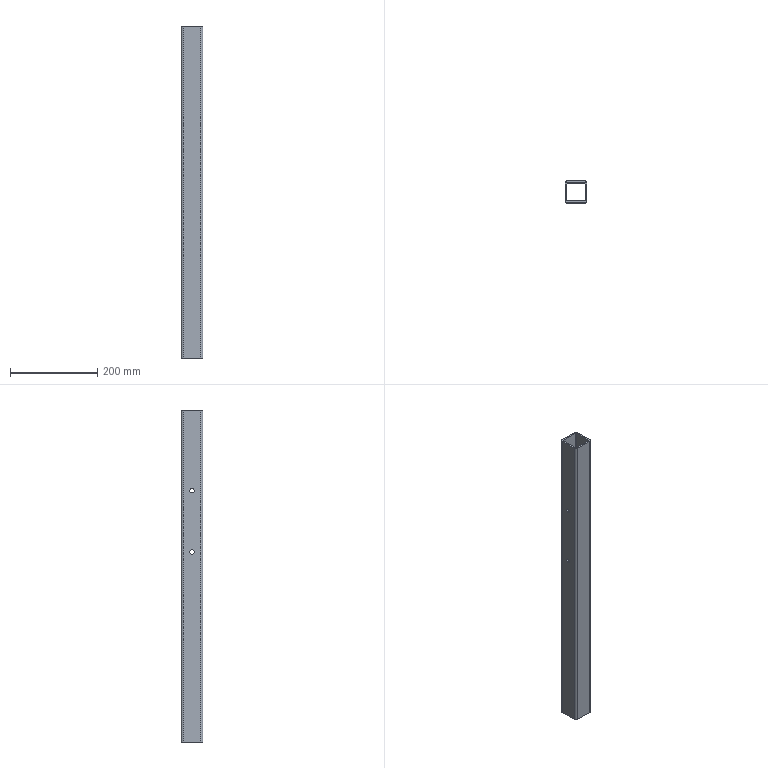Part | STEP file | 冲床-300配套压波_id1142_x_t | 1 solid | 22 faces | box 50 x 50 x 760 mm | volume 542446 mm3 | cylinder 12 | plane 10 | commonest cylinder face diameters 10 x8 2 x4
STEP:
#1=CARTESIAN_POINT('',(1916.,235.,-20.));
#2=VERTEX_POINT('',#1);
#3=CARTESIAN_POINT('',(1916.,275.,-20.));
#4=VERTEX_POINT('',#3);
#5=CARTESIAN_POINT('',(1916.,30.,-20.));
#6=DIRECTION('',(0.,1.,0.));
#7=VECTOR('',#6,1.);
#8=LINE('',#5,#7);
#9=EDGE_CURVE('',#2,#4,#8,.T.);
#10=ORIENTED_EDGE('',*,*,#9,.F.);
#11=CARTESIAN_POINT('',(1915.,234.,-20.));
#12=VERTEX_POINT('',#11);
#13=CARTESIAN_POINT('',(1915.,235.,-20.));
#14=DIRECTION('',(0.,0.,1.));
#15=DIRECTION('',(-1.,0.,0.));
#16=AXIS2_PLACEMENT_3D('',#13,#14,#15);
#17=CIRCLE('',#16,1.);
#18=EDGE_CURVE('',#12,#2,#17,.T.);
#19=ORIENTED_EDGE('',*,*,#18,.F.);
#20=CARTESIAN_POINT('',(1875.,234.,-20.));
#21=VERTEX_POINT('',#20);
#22=CARTESIAN_POINT('',(3070.,234.,-20.));
#23=DIRECTION('',(1.,0.,0.));
#24=VECTOR('',#23,1.);
#25=LINE('',#22,#24);
#26=EDGE_CURVE('',#21,#12,#25,.T.);
#27=ORIENTED_EDGE('',*,*,#26,.F.);
#28=CARTESIAN_POINT('',(1874.,235.,-20.));
#29=VERTEX_POINT('',#28);
#30=CARTESIAN_POINT('',(1875.,235.,-20.));
#31=DIRECTION('',(0.,0.,1.));
#32=DIRECTION('',(-1.,0.,0.));
#33=AXIS2_PLACEMENT_3D('',#30,#31,#32);
#34=CIRCLE('',#33,1.);
#35=EDGE_CURVE('',#29,#21,#34,.T.);
#36=ORIENTED_EDGE('',*,*,#35,.F.);
#37=CARTESIAN_POINT('',(1874.,275.,-20.));
#38=VERTEX_POINT('',#37);
#39=CARTESIAN_POINT('',(1874.,30.,-20.));
#40=DIRECTION('',(0.,-1.,0.));
#41=VECTOR('',#40,1.);
#42=LINE('',#39,#41);
#43=EDGE_CURVE('',#38,#29,#42,.T.);
#44=ORIENTED_EDGE('',*,*,#43,.F.);
#45=CARTESIAN_POINT('',(1875.,276.,-20.));
#46=VERTEX_POINT('',#45);
#47=CARTESIAN_POINT('',(1875.,275.,-20.));
#48=DIRECTION('',(0.,0.,1.));
#49=DIRECTION('',(-1.,0.,0.));
#50=AXIS2_PLACEMENT_3D('',#47,#48,#49);
#51=CIRCLE('',#50,1.);
#52=EDGE_CURVE('',#46,#38,#51,.T.);
#53=ORIENTED_EDGE('',*,*,#52,.F.);
#54=CARTESIAN_POINT('',(1915.,276.,-20.));
#55=VERTEX_POINT('',#54);
#56=CARTESIAN_POINT('',(3070.,276.,-20.));
#57=DIRECTION('',(-1.,0.,0.));
#58=VECTOR('',#57,1.);
#59=LINE('',#56,#58);
#60=EDGE_CURVE('',#55,#46,#59,.T.);
#61=ORIENTED_EDGE('',*,*,#60,.F.);
#62=CARTESIAN_POINT('',(1915.,275.,-20.));
#63=DIRECTION('',(0.,0.,1.));
#64=DIRECTION('',(-1.,0.,0.));
#65=AXIS2_PLACEMENT_3D('',#62,#63,#64);
#66=CIRCLE('',#65,1.);
#67=EDGE_CURVE('',#4,#55,#66,.T.);
#68=ORIENTED_EDGE('',*,*,#67,.F.);
#69=EDGE_LOOP('',(#10,#19,#27,#36,#44,#53,#61,#68));
#70=FACE_BOUND('',#69,.T.);
#71=CARTESIAN_POINT('',(1920.,235.,-20.));
#72=VERTEX_POINT('',#71);
#73=CARTESIAN_POINT('',(1920.,275.,-20.));
#74=VERTEX_POINT('',#73);
#75=CARTESIAN_POINT('',(1920.,275.,-20.));
#76=DIRECTION('',(0.,1.,0.));
#77=VECTOR('',#76,1.);
#78=LINE('',#75,#77);
#79=EDGE_CURVE('',#72,#74,#78,.T.);
#80=ORIENTED_EDGE('',*,*,#79,.T.);
#81=CARTESIAN_POINT('',(1915.,280.,-20.));
#82=VERTEX_POINT('',#81);
#83=CARTESIAN_POINT('',(1915.,275.,-20.));
#84=DIRECTION('',(0.,0.,1.));
#85=DIRECTION('',(-1.,0.,0.));
#86=AXIS2_PLACEMENT_3D('',#83,#84,#85);
#87=CIRCLE('',#86,5.);
#88=EDGE_CURVE('',#74,#82,#87,.T.);
#89=ORIENTED_EDGE('',*,*,#88,.T.);
#90=CARTESIAN_POINT('',(1875.,280.,-20.));
#91=VERTEX_POINT('',#90);
#92=CARTESIAN_POINT('',(1875.,280.,-20.));
#93=DIRECTION('',(-1.,0.,0.));
#94=VECTOR('',#93,1.);
#95=LINE('',#92,#94);
#96=EDGE_CURVE('',#82,#91,#95,.T.);
#97=ORIENTED_EDGE('',*,*,#96,.T.);
#98=CARTESIAN_POINT('',(1870.,275.,-20.));
#99=VERTEX_POINT('',#98);
#100=CARTESIAN_POINT('',(1875.,275.,-20.));
#101=DIRECTION('',(0.,0.,1.));
#102=DIRECTION('',(-1.,0.,0.));
#103=AXIS2_PLACEMENT_3D('',#100,#101,#102);
#104=CIRCLE('',#103,5.);
#105=EDGE_CURVE('',#91,#99,#104,.T.);
#106=ORIENTED_EDGE('',*,*,#105,.T.);
#107=CARTESIAN_POINT('',(1870.,235.,-20.));
#108=VERTEX_POINT('',#107);
#109=CARTESIAN_POINT('',(1870.,235.,-20.));
#110=DIRECTION('',(0.,-1.,0.));
#111=VECTOR('',#110,1.);
#112=LINE('',#109,#111);
#113=EDGE_CURVE('',#99,#108,#112,.T.);
#114=ORIENTED_EDGE('',*,*,#113,.T.);
#115=CARTESIAN_POINT('',(1875.,230.,-20.));
#116=VERTEX_POINT('',#115);
#117=CARTESIAN_POINT('',(1875.,235.,-20.));
#118=DIRECTION('',(0.,0.,1.));
#119=DIRECTION('',(-1.,0.,0.));
#120=AXIS2_PLACEMENT_3D('',#117,#118,#119);
#121=CIRCLE('',#120,5.);
#122=EDGE_CURVE('',#108,#116,#121,.T.);
#123=ORIENTED_EDGE('',*,*,#122,.T.);
#124=CARTESIAN_POINT('',(1915.,230.,-20.));
#125=VERTEX_POINT('',#124);
#126=CARTESIAN_POINT('',(1915.,230.,-20.));
#127=DIRECTION('',(1.,0.,0.));
#128=VECTOR('',#127,1.);
#129=LINE('',#126,#128);
#130=EDGE_CURVE('',#116,#125,#129,.T.);
#131=ORIENTED_EDGE('',*,*,#130,.T.);
#132=CARTESIAN_POINT('',(1915.,235.,-20.));
#133=DIRECTION('',(0.,0.,1.));
#134=DIRECTION('',(-1.,0.,0.));
#135=AXIS2_PLACEMENT_3D('',#132,#133,#134);
#136=CIRCLE('',#135,5.);
#137=EDGE_CURVE('',#125,#72,#136,.T.);
#138=ORIENTED_EDGE('',*,*,#137,.T.);
#139=EDGE_LOOP('',(#80,#89,#97,#106,#114,#123,#131,#138));
#140=FACE_BOUND('',#139,.T.);
#141=CARTESIAN_POINT('',(3070.,30.,-20.));
#142=DIRECTION('',(0.,0.,1.));
#143=DIRECTION('',(-1.,0.,0.));
#144=AXIS2_PLACEMENT_3D('',#141,#142,#143);
#145=PLANE('',#144);
#146=ADVANCED_FACE('',(#70,#140),#145,.T.);
#147=CARTESIAN_POINT('',(1915.,230.,-780.));
#148=VERTEX_POINT('',#147);
#149=CARTESIAN_POINT('',(1915.,230.,-740.));
#150=DIRECTION('',(0.,0.,-1.));
#151=VECTOR('',#150,1.);
#152=LINE('',#149,#151);
#153=EDGE_CURVE('',#125,#148,#152,.T.);
#154=ORIENTED_EDGE('',*,*,#153,.T.);
#155=CARTESIAN_POINT('',(1920.,235.,-780.));
#156=VERTEX_POINT('',#155);
#157=CARTESIAN_POINT('',(1915.,235.,-780.));
#158=DIRECTION('',(0.,0.,1.));
#159=DIRECTION('',(-1.,0.,0.));
#160=AXIS2_PLACEMENT_3D('',#157,#158,#159);
#161=CIRCLE('',#160,5.);
#162=EDGE_CURVE('',#148,#156,#161,.T.);
#163=ORIENTED_EDGE('',*,*,#162,.T.);
#164=CARTESIAN_POINT('',(1920.,235.,-740.));
#165=DIRECTION('',(0.,0.,-1.));
#166=VECTOR('',#165,1.);
#167=LINE('',#164,#166);
#168=EDGE_CURVE('',#72,#156,#167,.T.);
#169=ORIENTED_EDGE('',*,*,#168,.F.);
#170=ORIENTED_EDGE('',*,*,#137,.F.);
#171=EDGE_LOOP('',(#154,#163,#169,#170));
#172=FACE_OUTER_BOUND('',#171,.T.);
#173=CARTESIAN_POINT('',(1915.,235.,-740.));
#174=DIRECTION('',(0.,0.,1.));
#175=DIRECTION('',(-1.,0.,0.));
#176=AXIS2_PLACEMENT_3D('',#173,#174,#175);
#177=CYLINDRICAL_SURFACE('',#176,5.);
#178=ADVANCED_FACE('',(#172),#177,.T.);
#179=CARTESIAN_POINT('',(1875.,230.,-780.));
#180=VERTEX_POINT('',#179);
#181=CARTESIAN_POINT('',(1875.,230.,-740.));
#182=DIRECTION('',(0.,0.,-1.));
#183=VECTOR('',#182,1.);
#184=LINE('',#181,#183);
#185=EDGE_CURVE('',#116,#180,#184,.T.);
#186=ORIENTED_EDGE('',*,*,#185,.T.);
#187=CARTESIAN_POINT('',(1915.,230.,-780.));
#188=DIRECTION('',(1.,0.,0.));
#189=VECTOR('',#188,1.);
#190=LINE('',#187,#189);
#191=EDGE_CURVE('',#180,#148,#190,.T.);
#192=ORIENTED_EDGE('',*,*,#191,.T.);
#193=ORIENTED_EDGE('',*,*,#153,.F.);
#194=ORIENTED_EDGE('',*,*,#130,.F.);
#195=EDGE_LOOP('',(#186,#192,#193,#194));
#196=FACE_OUTER_BOUND('',#195,.T.);
#197=CARTESIAN_POINT('',(1915.,230.,-740.));
#198=DIRECTION('',(0.,-1.,0.));
#199=DIRECTION('',(-1.,0.,0.));
#200=AXIS2_PLACEMENT_3D('',#197,#198,#199);
#201=PLANE('',#200);
#202=ADVANCED_FACE('',(#196),#201,.T.);
#203=CARTESIAN_POINT('',(1870.,235.,-780.));
#204=VERTEX_POINT('',#203);
#205=CARTESIAN_POINT('',(1870.,235.,-740.));
#206=DIRECTION('',(0.,0.,-1.));
#207=VECTOR('',#206,1.);
#208=LINE('',#205,#207);
#209=EDGE_CURVE('',#108,#204,#208,.T.);
#210=ORIENTED_EDGE('',*,*,#209,.T.);
#211=CARTESIAN_POINT('',(1875.,235.,-780.));
#212=DIRECTION('',(0.,0.,1.));
#213=DIRECTION('',(-1.,0.,0.));
#214=AXIS2_PLACEMENT_3D('',#211,#212,#213);
#215=CIRCLE('',#214,5.);
#216=EDGE_CURVE('',#204,#180,#215,.T.);
#217=ORIENTED_EDGE('',*,*,#216,.T.);
#218=ORIENTED_EDGE('',*,*,#185,.F.);
#219=ORIENTED_EDGE('',*,*,#122,.F.);
#220=EDGE_LOOP('',(#210,#217,#218,#219));
#221=FACE_OUTER_BOUND('',#220,.T.);
#222=CARTESIAN_POINT('',(1875.,235.,-740.));
#223=DIRECTION('',(0.,0.,1.));
#224=DIRECTION('',(-1.,0.,0.));
#225=AXIS2_PLACEMENT_3D('',#222,#223,#224);
#226=CYLINDRICAL_SURFACE('',#225,5.);
#227=ADVANCED_FACE('',(#221),#226,.T.);
#228=CARTESIAN_POINT('',(1870.,255.,-340.));
#229=VERTEX_POINT('',#228);
#230=CARTESIAN_POINT('',(1870.,255.,-345.));
#231=DIRECTION('',(1.,0.,0.));
#232=DIRECTION('',(0.,0.,1.));
#233=AXIS2_PLACEMENT_3D('',#230,#231,#232);
#234=CIRCLE('',#233,5.);
#235=EDGE_CURVE('',#229,#229,#234,.T.);
#236=ORIENTED_EDGE('',*,*,#235,.T.);
#237=EDGE_LOOP('',(#236));
#238=FACE_BOUND('',#237,.T.);
#239=CARTESIAN_POINT('',(1870.,255.,-200.));
#240=VERTEX_POINT('',#239);
#241=CARTESIAN_POINT('',(1870.,255.,-205.));
#242=DIRECTION('',(1.,0.,0.));
#243=DIRECTION('',(0.,0.,1.));
#244=AXIS2_PLACEMENT_3D('',#241,#242,#243);
#245=CIRCLE('',#244,5.);
#246=EDGE_CURVE('',#240,#240,#245,.T.);
#247=ORIENTED_EDGE('',*,*,#246,.T.);
#248=EDGE_LOOP('',(#247));
#249=FACE_BOUND('',#248,.T.);
#250=CARTESIAN_POINT('',(1870.,275.,-780.));
#251=VERTEX_POINT('',#250);
#252=CARTESIAN_POINT('',(1870.,275.,-740.));
#253=DIRECTION('',(0.,0.,-1.));
#254=VECTOR('',#253,1.);
#255=LINE('',#252,#254);
#256=EDGE_CURVE('',#99,#251,#255,.T.);
#257=ORIENTED_EDGE('',*,*,#256,.T.);
#258=CARTESIAN_POINT('',(1870.,235.,-780.));
#259=DIRECTION('',(0.,-1.,0.));
#260=VECTOR('',#259,1.);
#261=LINE('',#258,#260);
#262=EDGE_CURVE('',#251,#204,#261,.T.);
#263=ORIENTED_EDGE('',*,*,#262,.T.);
#264=ORIENTED_EDGE('',*,*,#209,.F.);
#265=ORIENTED_EDGE('',*,*,#113,.F.);
#266=EDGE_LOOP('',(#257,#263,#264,#265));
#267=FACE_BOUND('',#266,.T.);
#268=CARTESIAN_POINT('',(1870.,235.,-740.));
#269=DIRECTION('',(-1.,0.,0.));
#270=DIRECTION('',(0.,0.,-1.));
#271=AXIS2_PLACEMENT_3D('',#268,#269,#270);
#272=PLANE('',#271);
#273=ADVANCED_FACE('',(#238,#249,#267),#272,.T.);
#274=CARTESIAN_POINT('',(1875.,280.,-780.));
#275=VERTEX_POINT('',#274);
#276=CARTESIAN_POINT('',(1875.,280.,-740.));
#277=DIRECTION('',(0.,0.,-1.));
#278=VECTOR('',#277,1.);
#279=LINE('',#276,#278);
#280=EDGE_CURVE('',#91,#275,#279,.T.);
#281=ORIENTED_EDGE('',*,*,#280,.T.);
#282=CARTESIAN_POINT('',(1875.,275.,-780.));
#283=DIRECTION('',(0.,0.,1.));
#284=DIRECTION('',(-1.,0.,0.));
#285=AXIS2_PLACEMENT_3D('',#282,#283,#284);
#286=CIRCLE('',#285,5.);
#287=EDGE_CURVE('',#275,#251,#286,.T.);
#288=ORIENTED_EDGE('',*,*,#287,.T.);
#289=ORIENTED_EDGE('',*,*,#256,.F.);
#290=ORIENTED_EDGE('',*,*,#105,.F.);
#291=EDGE_LOOP('',(#281,#288,#289,#290));
#292=FACE_OUTER_BOUND('',#291,.T.);
#293=CARTESIAN_POINT('',(1875.,275.,-740.));
#294=DIRECTION('',(0.,0.,1.));
#295=DIRECTION('',(-1.,0.,0.));
#296=AXIS2_PLACEMENT_3D('',#293,#294,#295);
#297=CYLINDRICAL_SURFACE('',#296,5.);
#298=ADVANCED_FACE('',(#292),#297,.T.);
#299=CARTESIAN_POINT('',(1916.,275.,-780.));
#300=VERTEX_POINT('',#299);
#301=CARTESIAN_POINT('',(1915.,276.,-780.));
#302=VERTEX_POINT('',#301);
#303=CARTESIAN_POINT('',(1915.,275.,-780.));
#304=DIRECTION('',(0.,0.,1.));
#305=DIRECTION('',(-1.,0.,0.));
#306=AXIS2_PLACEMENT_3D('',#303,#304,#305);
#307=CIRCLE('',#306,1.);
#308=EDGE_CURVE('',#300,#302,#307,.T.);
#309=ORIENTED_EDGE('',*,*,#308,.T.);
#310=CARTESIAN_POINT('',(1875.,276.,-780.));
#311=VERTEX_POINT('',#310);
#312=CARTESIAN_POINT('',(1915.,276.,-780.));
#313=DIRECTION('',(-1.,0.,0.));
#314=VECTOR('',#313,1.);
#315=LINE('',#312,#314);
#316=EDGE_CURVE('',#302,#311,#315,.T.);
#317=ORIENTED_EDGE('',*,*,#316,.T.);
#318=CARTESIAN_POINT('',(1874.,275.,-780.));
#319=VERTEX_POINT('',#318);
#320=CARTESIAN_POINT('',(1875.,275.,-780.));
#321=DIRECTION('',(0.,0.,1.));
#322=DIRECTION('',(-1.,0.,0.));
#323=AXIS2_PLACEMENT_3D('',#320,#321,#322);
#324=CIRCLE('',#323,1.);
#325=EDGE_CURVE('',#311,#319,#324,.T.);
#326=ORIENTED_EDGE('',*,*,#325,.T.);
#327=CARTESIAN_POINT('',(1874.,235.,-780.));
#328=VERTEX_POINT('',#327);
#329=CARTESIAN_POINT('',(1874.,235.,-780.));
#330=DIRECTION('',(0.,-1.,0.));
#331=VECTOR('',#330,1.);
#332=LINE('',#329,#331);
#333=EDGE_CURVE('',#319,#328,#332,.T.);
#334=ORIENTED_EDGE('',*,*,#333,.T.);
#335=CARTESIAN_POINT('',(1875.,234.,-780.));
#336=VERTEX_POINT('',#335);
#337=CARTESIAN_POINT('',(1875.,235.,-780.));
#338=DIRECTION('',(0.,0.,1.));
#339=DIRECTION('',(-1.,0.,0.));
#340=AXIS2_PLACEMENT_3D('',#337,#338,#339);
#341=CIRCLE('',#340,1.);
#342=EDGE_CURVE('',#328,#336,#341,.T.);
#343=ORIENTED_EDGE('',*,*,#342,.T.);
#344=CARTESIAN_POINT('',(1915.,234.,-780.));
#345=VERTEX_POINT('',#344);
#346=CARTESIAN_POINT('',(1915.,234.,-780.));
#347=DIRECTION('',(1.,0.,0.));
#348=VECTOR('',#347,1.);
#349=LINE('',#346,#348);
#350=EDGE_CURVE('',#336,#345,#349,.T.);
#351=ORIENTED_EDGE('',*,*,#350,.T.);
#352=CARTESIAN_POINT('',(1916.,235.,-780.));
#353=VERTEX_POINT('',#352);
#354=CARTESIAN_POINT('',(1915.,235.,-780.));
#355=DIRECTION('',(0.,0.,1.));
#356=DIRECTION('',(-1.,0.,0.));
#357=AXIS2_PLACEMENT_3D('',#354,#355,#356);
#358=CIRCLE('',#357,1.);
#359=EDGE_CURVE('',#345,#353,#358,.T.);
#360=ORIENTED_EDGE('',*,*,#359,.T.);
#361=CARTESIAN_POINT('',(1916.,235.,-780.));
#362=DIRECTION('',(0.,1.,0.));
#363=VECTOR('',#362,1.);
#364=LINE('',#361,#363);
#365=EDGE_CURVE('',#353,#300,#364,.T.);
#366=ORIENTED_EDGE('',*,*,#365,.T.);
#367=EDGE_LOOP('',(#309,#317,#326,#334,#343,#351,#360,#366));
#368=FACE_BOUND('',#367,.T.);
#369=CARTESIAN_POINT('',(1920.,275.,-780.));
#370=VERTEX_POINT('',#369);
#371=CARTESIAN_POINT('',(1920.,235.,-780.));
#372=DIRECTION('',(0.,1.,0.));
#373=VECTOR('',#372,1.);
#374=LINE('',#371,#373);
#375=EDGE_CURVE('',#156,#370,#374,.T.);
#376=ORIENTED_EDGE('',*,*,#375,.F.);
#377=ORIENTED_EDGE('',*,*,#162,.F.);
#378=ORIENTED_EDGE('',*,*,#191,.F.);
#379=ORIENTED_EDGE('',*,*,#216,.F.);
#380=ORIENTED_EDGE('',*,*,#262,.F.);
#381=ORIENTED_EDGE('',*,*,#287,.F.);
#382=CARTESIAN_POINT('',(1915.,280.,-780.));
#383=VERTEX_POINT('',#382);
#384=CARTESIAN_POINT('',(1915.,280.,-780.));
#385=DIRECTION('',(-1.,0.,0.));
#386=VECTOR('',#385,1.);
#387=LINE('',#384,#386);
#388=EDGE_CURVE('',#383,#275,#387,.T.);
#389=ORIENTED_EDGE('',*,*,#388,.F.);
#390=CARTESIAN_POINT('',(1915.,275.,-780.));
#391=DIRECTION('',(0.,0.,1.));
#392=DIRECTION('',(-1.,0.,0.));
#393=AXIS2_PLACEMENT_3D('',#390,#391,#392);
#394=CIRCLE('',#393,5.);
#395=EDGE_CURVE('',#370,#383,#394,.T.);
#396=ORIENTED_EDGE('',*,*,#395,.F.);
#397=EDGE_LOOP('',(#376,#377,#378,#379,#380,#381,#389,#396));
#398=FACE_BOUND('',#397,.T.);
#399=CARTESIAN_POINT('',(1915.,235.,-780.));
#400=DIRECTION('',(0.,0.,1.));
#401=DIRECTION('',(-1.,0.,0.));
#402=AXIS2_PLACEMENT_3D('',#399,#400,#401);
#403=PLANE('',#402);
#404=ADVANCED_FACE('',(#368,#398),#403,.F.);
#405=CARTESIAN_POINT('',(1915.,280.,-740.));
#406=DIRECTION('',(0.,0.,-1.));
#407=VECTOR('',#406,1.);
#408=LINE('',#405,#407);
#409=EDGE_CURVE('',#82,#383,#408,.T.);
#410=ORIENTED_EDGE('',*,*,#409,.T.);
#411=ORIENTED_EDGE('',*,*,#388,.T.);
#412=ORIENTED_EDGE('',*,*,#280,.F.);
#413=ORIENTED_EDGE('',*,*,#96,.F.);
#414=EDGE_LOOP('',(#410,#411,#412,#413));
#415=FACE_OUTER_BOUND('',#414,.T.);
#416=CARTESIAN_POINT('',(1875.,280.,-740.));
#417=DIRECTION('',(0.,1.,0.));
#418=DIRECTION('',(1.,0.,0.));
#419=AXIS2_PLACEMENT_3D('',#416,#417,#418);
#420=PLANE('',#419);
#421=ADVANCED_FACE('',(#415),#420,.T.);
#422=CARTESIAN_POINT('',(1920.,255.,-350.));
#423=VERTEX_POINT('',#422);
#424=CARTESIAN_POINT('',(1920.,255.,-345.));
#425=DIRECTION('',(-1.,0.,0.));
#426=DIRECTION('',(0.,0.,-1.));
#427=AXIS2_PLACEMENT_3D('',#424,#425,#426);
#428=CIRCLE('',#427,5.);
#429=EDGE_CURVE('',#423,#423,#428,.T.);
#430=ORIENTED_EDGE('',*,*,#429,.T.);
#431=EDGE_LOOP('',(#430));
#432=FACE_BOUND('',#431,.T.);
#433=CARTESIAN_POINT('',(1920.,255.,-210.));
#434=VERTEX_POINT('',#433);
#435=CARTESIAN_POINT('',(1920.,255.,-205.));
#436=DIRECTION('',(-1.,0.,0.));
#437=DIRECTION('',(0.,0.,-1.));
#438=AXIS2_PLACEMENT_3D('',#435,#436,#437);
#439=CIRCLE('',#438,5.);
#440=EDGE_CURVE('',#434,#434,#439,.T.);
#441=ORIENTED_EDGE('',*,*,#440,.T.);
#442=EDGE_LOOP('',(#441));
#443=FACE_BOUND('',#442,.T.);
#444=ORIENTED_EDGE('',*,*,#168,.T.);
#445=ORIENTED_EDGE('',*,*,#375,.T.);
#446=CARTESIAN_POINT('',(1920.,275.,-740.));
#447=DIRECTION('',(0.,0.,-1.));
#448=VECTOR('',#447,1.);
#449=LINE('',#446,#448);
#450=EDGE_CURVE('',#74,#370,#449,.T.);
#451=ORIENTED_EDGE('',*,*,#450,.F.);
#452=ORIENTED_EDGE('',*,*,#79,.F.);
#453=EDGE_LOOP('',(#444,#445,#451,#452));
#454=FACE_BOUND('',#453,.T.);
#455=CARTESIAN_POINT('',(1920.,275.,-740.));
#456=DIRECTION('',(1.,0.,0.));
#457=DIRECTION('',(0.,0.,1.));
#458=AXIS2_PLACEMENT_3D('',#455,#456,#457);
#459=PLANE('',#458);
#460=ADVANCED_FACE('',(#432,#443,#454),#459,.T.);
#461=ORIENTED_EDGE('',*,*,#450,.T.);
#462=ORIENTED_EDGE('',*,*,#395,.T.);
#463=ORIENTED_EDGE('',*,*,#409,.F.);
#464=ORIENTED_EDGE('',*,*,#88,.F.);
#465=EDGE_LOOP('',(#461,#462,#463,#464));
#466=FACE_OUTER_BOUND('',#465,.T.);
#467=CARTESIAN_POINT('',(1915.,275.,-740.));
#468=DIRECTION('',(0.,0.,1.));
#469=DIRECTION('',(-1.,0.,0.));
#470=AXIS2_PLACEMENT_3D('',#467,#468,#469);
#471=CYLINDRICAL_SURFACE('',#470,5.);
#472=ADVANCED_FACE('',(#466),#471,.T.);
#473=CARTESIAN_POINT('',(1915.,234.,-740.));
#474=DIRECTION('',(0.,0.,-1.));
#475=VECTOR('',#474,1.);
#476=LINE('',#473,#475);
#477=EDGE_CURVE('',#12,#345,#476,.T.);
#478=ORIENTED_EDGE('',*,*,#477,.F.);
#479=ORIENTED_EDGE('',*,*,#18,.T.);
#480=CARTESIAN_POINT('',(1916.,235.,-740.));
#481=DIRECTION('',(0.,0.,-1.));
#482=VECTOR('',#481,1.);
#483=LINE('',#480,#482);
#484=EDGE_CURVE('',#2,#353,#483,.T.);
#485=ORIENTED_EDGE('',*,*,#484,.T.);
#486=ORIENTED_EDGE('',*,*,#359,.F.);
#487=EDGE_LOOP('',(#478,#479,#485,#486));
#488=FACE_OUTER_BOUND('',#487,.T.);
#489=CARTESIAN_POINT('',(1915.,235.,-740.));
#490=DIRECTION('',(0.,0.,1.));
#491=DIRECTION('',(-1.,0.,0.));
#492=AXIS2_PLACEMENT_3D('',#489,#490,#491);
#493=CYLINDRICAL_SURFACE('',#492,1.);
#494=ADVANCED_FACE('',(#488),#493,.F.);
#495=CARTESIAN_POINT('',(1875.,234.,-740.));
#496=DIRECTION('',(0.,0.,-1.));
#497=VECTOR('',#496,1.);
#498=LINE('',#495,#497);
#499=EDGE_CURVE('',#21,#336,#498,.T.);
#500=ORIENTED_EDGE('',*,*,#499,.F.);
#501=ORIENTED_EDGE('',*,*,#26,.T.);
#502=ORIENTED_EDGE('',*,*,#477,.T.);
#503=ORIENTED_EDGE('',*,*,#350,.F.);
#504=EDGE_LOOP('',(#500,#501,#502,#503));
#505=FACE_OUTER_BOUND('',#504,.T.);
#506=CARTESIAN_POINT('',(1915.,234.,-740.));
#507=DIRECTION('',(0.,-1.,0.));
#508=DIRECTION('',(-1.,0.,0.));
#509=AXIS2_PLACEMENT_3D('',#506,#507,#508);
#510=PLANE('',#509);
#511=ADVANCED_FACE('',(#505),#510,.F.);
#512=CARTESIAN_POINT('',(1874.,235.,-740.));
#513=DIRECTION('',(0.,0.,-1.));
#514=VECTOR('',#513,1.);
#515=LINE('',#512,#514);
#516=EDGE_CURVE('',#29,#328,#515,.T.);
#517=ORIENTED_EDGE('',*,*,#516,.F.);
#518=ORIENTED_EDGE('',*,*,#35,.T.);
#519=ORIENTED_EDGE('',*,*,#499,.T.);
#520=ORIENTED_EDGE('',*,*,#342,.F.);
#521=EDGE_LOOP('',(#517,#518,#519,#520));
#522=FACE_OUTER_BOUND('',#521,.T.);
#523=CARTESIAN_POINT('',(1875.,235.,-740.));
#524=DIRECTION('',(0.,0.,1.));
#525=DIRECTION('',(-1.,0.,0.));
#526=AXIS2_PLACEMENT_3D('',#523,#524,#525);
#527=CYLINDRICAL_SURFACE('',#526,1.);
#528=ADVANCED_FACE('',(#522),#527,.F.);
#529=CARTESIAN_POINT('',(1874.,255.,-340.));
#530=VERTEX_POINT('',#529);
#531=CARTESIAN_POINT('',(1874.,255.,-345.));
#532=DIRECTION('',(1.,0.,0.));
#533=DIRECTION('',(0.,0.,1.));
#534=AXIS2_PLACEMENT_3D('',#531,#532,#533);
#535=CIRCLE('',#534,5.);
#536=EDGE_CURVE('',#530,#530,#535,.T.);
#537=ORIENTED_EDGE('',*,*,#536,.F.);
#538=EDGE_LOOP('',(#537));
#539=FACE_BOUND('',#538,.T.);
#540=CARTESIAN_POINT('',(1874.,255.,-200.));
#541=VERTEX_POINT('',#540);
#542=CARTESIAN_POINT('',(1874.,255.,-205.));
#543=DIRECTION('',(1.,0.,0.));
#544=DIRECTION('',(0.,0.,1.));
#545=AXIS2_PLACEMENT_3D('',#542,#543,#544);
#546=CIRCLE('',#545,5.);
#547=EDGE_CURVE('',#541,#541,#546,.T.);
#548=ORIENTED_EDGE('',*,*,#547,.F.);
#549=EDGE_LOOP('',(#548));
#550=FACE_BOUND('',#549,.T.);
#551=CARTESIAN_POINT('',(1874.,275.,-740.));
#552=DIRECTION('',(0.,0.,-1.));
#553=VECTOR('',#552,1.);
#554=LINE('',#551,#553);
#555=EDGE_CURVE('',#38,#319,#554,.T.);
#556=ORIENTED_EDGE('',*,*,#555,.F.);
#557=ORIENTED_EDGE('',*,*,#43,.T.);
#558=ORIENTED_EDGE('',*,*,#516,.T.);
#559=ORIENTED_EDGE('',*,*,#333,.F.);
#560=EDGE_LOOP('',(#556,#557,#558,#559));
#561=FACE_BOUND('',#560,.T.);
#562=CARTESIAN_POINT('',(1874.,235.,-740.));
#563=DIRECTION('',(-1.,0.,0.));
#564=DIRECTION('',(0.,0.,-1.));
#565=AXIS2_PLACEMENT_3D('',#562,#563,#564);
#566=PLANE('',#565);
#567=ADVANCED_FACE('',(#539,#550,#561),#566,.F.);
#568=CARTESIAN_POINT('',(1875.,276.,-740.));
#569=DIRECTION('',(0.,0.,-1.));
#570=VECTOR('',#569,1.);
#571=LINE('',#568,#570);
#572=EDGE_CURVE('',#46,#311,#571,.T.);
#573=ORIENTED_EDGE('',*,*,#572,.F.);
#574=ORIENTED_EDGE('',*,*,#52,.T.);
#575=ORIENTED_EDGE('',*,*,#555,.T.);
#576=ORIENTED_EDGE('',*,*,#325,.F.);
#577=EDGE_LOOP('',(#573,#574,#575,#576));
#578=FACE_OUTER_BOUND('',#577,.T.);
#579=CARTESIAN_POINT('',(1875.,275.,-740.));
#580=DIRECTION('',(0.,0.,1.));
#581=DIRECTION('',(-1.,0.,0.));
#582=AXIS2_PLACEMENT_3D('',#579,#580,#581);
#583=CYLINDRICAL_SURFACE('',#582,1.);
#584=ADVANCED_FACE('',(#578),#583,.F.);
#585=CARTESIAN_POINT('',(1915.,276.,-740.));
#586=DIRECTION('',(0.,0.,-1.));
#587=VECTOR('',#586,1.);
#588=LINE('',#585,#587);
#589=EDGE_CURVE('',#55,#302,#588,.T.);
#590=ORIENTED_EDGE('',*,*,#589,.F.);
#591=ORIENTED_EDGE('',*,*,#60,.T.);
#592=ORIENTED_EDGE('',*,*,#572,.T.);
#593=ORIENTED_EDGE('',*,*,#316,.F.);
#594=EDGE_LOOP('',(#590,#591,#592,#593));
#595=FACE_OUTER_BOUND('',#594,.T.);
#596=CARTESIAN_POINT('',(1875.,276.,-740.));
#597=DIRECTION('',(0.,1.,0.));
#598=DIRECTION('',(1.,0.,0.));
#599=AXIS2_PLACEMENT_3D('',#596,#597,#598);
#600=PLANE('',#599);
#601=ADVANCED_FACE('',(#595),#600,.F.);
#602=CARTESIAN_POINT('',(1916.,255.,-350.));
#603=VERTEX_POINT('',#602);
#604=CARTESIAN_POINT('',(1916.,255.,-345.));
#605=DIRECTION('',(-1.,0.,0.));
#606=DIRECTION('',(0.,0.,-1.));
#607=AXIS2_PLACEMENT_3D('',#604,#605,#606);
#608=CIRCLE('',#607,5.);
#609=EDGE_CURVE('',#603,#603,#608,.T.);
#610=ORIENTED_EDGE('',*,*,#609,.F.);
#611=EDGE_LOOP('',(#610));
#612=FACE_BOUND('',#611,.T.);
#613=CARTESIAN_POINT('',(1916.,255.,-210.));
#614=VERTEX_POINT('',#613);
#615=CARTESIAN_POINT('',(1916.,255.,-205.));
#616=DIRECTION('',(-1.,0.,0.));
#617=DIRECTION('',(0.,0.,-1.));
#618=AXIS2_PLACEMENT_3D('',#615,#616,#617);
#619=CIRCLE('',#618,5.);
#620=EDGE_CURVE('',#614,#614,#619,.T.);
#621=ORIENTED_EDGE('',*,*,#620,.F.);
#622=EDGE_LOOP('',(#621));
#623=FACE_BOUND('',#622,.T.);
#624=ORIENTED_EDGE('',*,*,#484,.F.);
#625=ORIENTED_EDGE('',*,*,#9,.T.);
#626=CARTESIAN_POINT('',(1916.,275.,-740.));
#627=DIRECTION('',(0.,0.,-1.));
#628=VECTOR('',#627,1.);
#629=LINE('',#626,#628);
#630=EDGE_CURVE('',#4,#300,#629,.T.);
#631=ORIENTED_EDGE('',*,*,#630,.T.);
#632=ORIENTED_EDGE('',*,*,#365,.F.);
#633=EDGE_LOOP('',(#624,#625,#631,#632));
#634=FACE_BOUND('',#633,.T.);
#635=CARTESIAN_POINT('',(1916.,275.,-740.));
#636=DIRECTION('',(1.,0.,0.));
#637=DIRECTION('',(0.,0.,1.));
#638=AXIS2_PLACEMENT_3D('',#635,#636,#637);
#639=PLANE('',#638);
#640=ADVANCED_FACE('',(#612,#623,#634),#639,.F.);
#641=ORIENTED_EDGE('',*,*,#630,.F.);
#642=ORIENTED_EDGE('',*,*,#67,.T.);
#643=ORIENTED_EDGE('',*,*,#589,.T.);
#644=ORIENTED_EDGE('',*,*,#308,.F.);
#645=EDGE_LOOP('',(#641,#642,#643,#644));
#646=FACE_OUTER_BOUND('',#645,.T.);
#647=CARTESIAN_POINT('',(1915.,275.,-740.));
#648=DIRECTION('',(0.,0.,1.));
#649=DIRECTION('',(-1.,0.,0.));
#650=AXIS2_PLACEMENT_3D('',#647,#648,#649);
#651=CYLINDRICAL_SURFACE('',#650,1.);
#652=ADVANCED_FACE('',(#646),#651,.F.);
#653=ORIENTED_EDGE('',*,*,#440,.F.);
#654=EDGE_LOOP('',(#653));
#655=FACE_BOUND('',#654,.T.);
#656=ORIENTED_EDGE('',*,*,#620,.T.);
#657=EDGE_LOOP('',(#656));
#658=FACE_BOUND('',#657,.T.);
#659=CARTESIAN_POINT('',(2085.,255.,-205.));
#660=DIRECTION('',(-1.,0.,0.));
#661=DIRECTION('',(0.,0.,-1.));
#662=AXIS2_PLACEMENT_3D('',#659,#660,#661);
#663=CYLINDRICAL_SURFACE('',#662,5.);
#664=ADVANCED_FACE('',(#655,#658),#663,.F.);
#665=ORIENTED_EDGE('',*,*,#429,.F.);
#666=EDGE_LOOP('',(#665));
#667=FACE_BOUND('',#666,.T.);
#668=ORIENTED_EDGE('',*,*,#609,.T.);
#669=EDGE_LOOP('',(#668));
#670=FACE_BOUND('',#669,.T.);
#671=CARTESIAN_POINT('',(2085.,255.,-345.));
#672=DIRECTION('',(-1.,0.,0.));
#673=DIRECTION('',(0.,0.,1.));
#674=AXIS2_PLACEMENT_3D('',#671,#672,#673);
#675=CYLINDRICAL_SURFACE('',#674,5.);
#676=ADVANCED_FACE('',(#667,#670),#675,.F.);
#677=ORIENTED_EDGE('',*,*,#246,.F.);
#678=EDGE_LOOP('',(#677));
#679=FACE_BOUND('',#678,.T.);
#680=ORIENTED_EDGE('',*,*,#547,.T.);
#681=EDGE_LOOP('',(#680));
#682=FACE_BOUND('',#681,.T.);
#683=CARTESIAN_POINT('',(2085.,255.,-205.));
#684=DIRECTION('',(-1.,0.,0.));
#685=DIRECTION('',(0.,0.,-1.));
#686=AXIS2_PLACEMENT_3D('',#683,#684,#685);
#687=CYLINDRICAL_SURFACE('',#686,5.);
#688=ADVANCED_FACE('',(#679,#682),#687,.F.);
#689=ORIENTED_EDGE('',*,*,#235,.F.);
#690=EDGE_LOOP('',(#689));
#691=FACE_BOUND('',#690,.T.);
#692=ORIENTED_EDGE('',*,*,#536,.T.);
#693=EDGE_LOOP('',(#692));
#694=FACE_BOUND('',#693,.T.);
#695=CARTESIAN_POINT('',(2085.,255.,-345.));
#696=DIRECTION('',(-1.,0.,0.));
#697=DIRECTION('',(0.,0.,1.));
#698=AXIS2_PLACEMENT_3D('',#695,#696,#697);
#699=CYLINDRICAL_SURFACE('',#698,5.);
#700=ADVANCED_FACE('',(#691,#694),#699,.F.);
#701=CLOSED_SHELL('',(#146,#178,#202,#227,#273,#298,#404,#421,#460,#472,#494,#511,#528,#567,#584,#601,#640,#652,#664,#676,#688,#700));
#702=MANIFOLD_SOLID_BREP('',#701);
#703=(LENGTH_UNIT()NAMED_UNIT(*)SI_UNIT(.MILLI.,.METRE.));
#704=UNCERTAINTY_MEASURE_WITH_UNIT(LENGTH_MEASURE(0.00002),#703,'','');
#705=(NAMED_UNIT(*)PLANE_ANGLE_UNIT()SI_UNIT($,.RADIAN.));
#706=PLANE_ANGLE_MEASURE_WITH_UNIT(PLANE_ANGLE_MEASURE(0.01745),#705);
#707=DIMENSIONAL_EXPONENTS(0.,0.,0.,0.,0.,0.,0.);
#708=(CONVERSION_BASED_UNIT('DEGREE',#706)NAMED_UNIT(#707)PLANE_ANGLE_UNIT());
#709=(NAMED_UNIT(*)SI_UNIT($,.STERADIAN.)SOLID_ANGLE_UNIT());
#710=(GEOMETRIC_REPRESENTATION_CONTEXT(3)GLOBAL_UNCERTAINTY_ASSIGNED_CONTEXT((#704))GLOBAL_UNIT_ASSIGNED_CONTEXT((#703,#708,#709))REPRESENTATION_CONTEXT('',''));
#711=ADVANCED_BREP_SHAPE_REPRESENTATION('',(#702),#710);